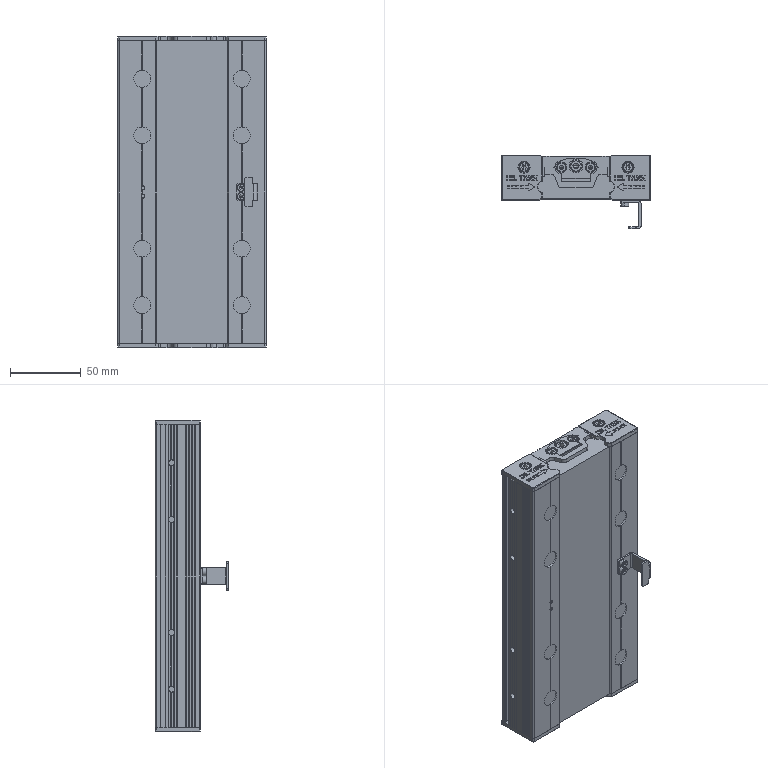Part | SolidWorks | features BaseBody 3 | 3 solids | 2162 faces | box 105 x 52 x 220 mm | volume 691685 mm3 | plane 1293 | cylinder 600 | cone 193 | torus 44 | spline 32 | commonest cylinder face diameters 0.2 x152 0.4 x95 2 x38 4.2 x36 7 x36 8 x25